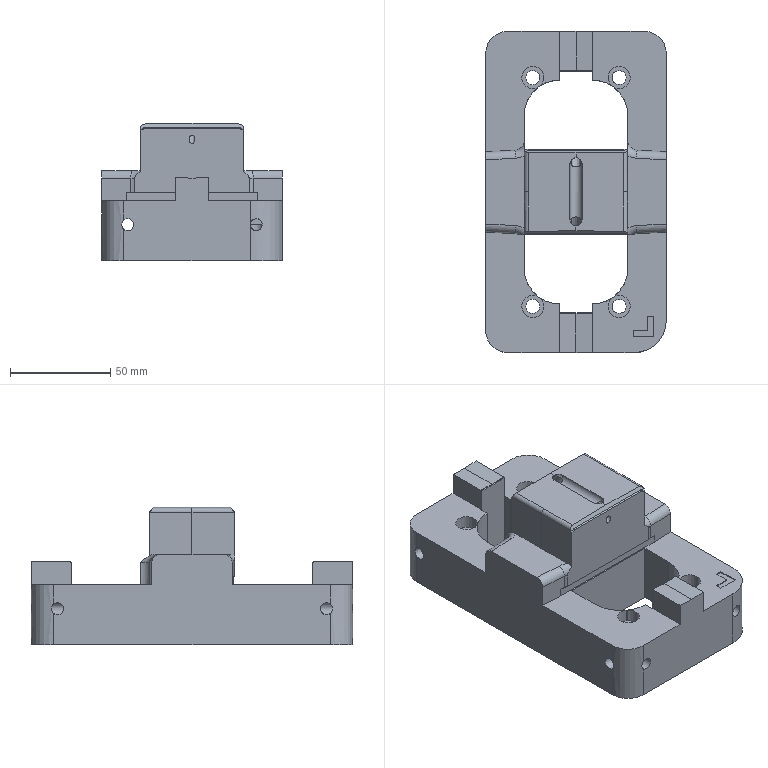Part | STEP file | lll_id106_x_t | 1 solid | 148 faces | box 90 x 160 x 68.59 mm | volume 417542 mm3 | plane 70 | cylinder 54 | spline 12 | cone 6 | torus 4 | sphere 2 | commonest cylinder face diameters 6 x12 6.8 x8 0.602 x4 4.016 x4 7 x4 8 x4